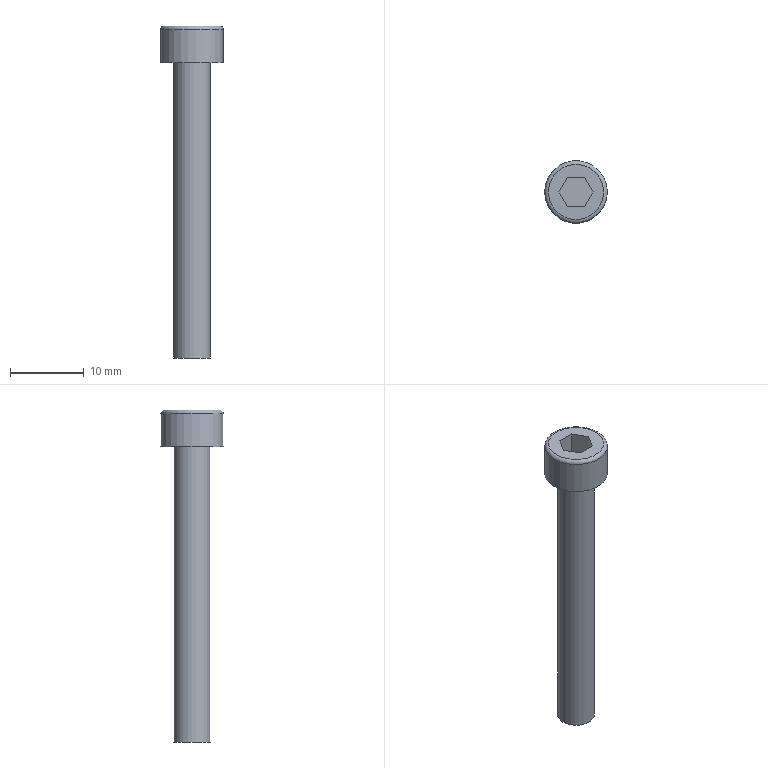Part | STEP file | Tube necking machine_id750_x_t | 1 solid | 13 faces | box 8.5 x 8.5 x 45 mm | volume 1022 mm3 | plane 10 | cylinder 2 | torus 1 | commonest cylinder face diameters 5 x1 8.5 x1
STEP:
#1=CARTESIAN_POINT('',(0.,0.,0.));
#2=DIRECTION('',(0.,0.,1.));
#3=DIRECTION('',(1.,0.,0.));
#4=AXIS2_PLACEMENT_3D('',#1,#2,#3);
#5=CARTESIAN_POINT('',(-17.75,-335.,207.));
#6=VERTEX_POINT('',#5);
#7=CARTESIAN_POINT('',(-14.,-335.,207.));
#8=DIRECTION('',(0.,0.,1.));
#9=DIRECTION('',(-1.,0.,0.));
#10=AXIS2_PLACEMENT_3D('',#7,#8,#9);
#11=CIRCLE('',#10,3.75);
#12=CARTESIAN_POINT('',(-9.75,-335.,207.));
#13=DIRECTION('',(0.,0.,-1.));
#14=DIRECTION('',(-1.,0.,0.));
#15=AXIS2_PLACEMENT_3D('',#12,#13,#14);
#16=PLANE('',#15);
#17=CARTESIAN_POINT('',(8.,0.));
#18=CARTESIAN_POINT('',(8.,-6.495));
#19=CARTESIAN_POINT('',(2.375,-3.248));
#20=CARTESIAN_POINT('',(-3.25,0.));
#21=CARTESIAN_POINT('',(2.375,3.248));
#22=CARTESIAN_POINT('',(8.,6.495));
#23=CARTESIAN_POINT('',(8.,0.));
#24=(BOUNDED_CURVE()B_SPLINE_CURVE(2,(#17,#18,#19,#20,#21,#22,#23),.UNSPECIFIED.,.T.,.F.)B_SPLINE_CURVE_WITH_KNOTS((1,2,2,2,2,1),(-2.094,0.,2.094,4.189,6.283,8.378),.UNSPECIFIED.)CURVE()GEOMETRIC_REPRESENTATION_ITEM()RATIONAL_B_SPLINE_CURVE((1.,0.5,1.,0.5,1.,0.5,1.))REPRESENTATION_ITEM(''));
#25=(GEOMETRIC_REPRESENTATION_CONTEXT(2)PARAMETRIC_REPRESENTATION_CONTEXT()REPRESENTATION_CONTEXT('',''));
#26=DEFINITIONAL_REPRESENTATION('',(#24),#25);
#27=PCURVE('',#16,#26);
#28=CARTESIAN_POINT('',(-14.,-335.,206.5));
#29=DIRECTION('',(0.,0.,-1.));
#30=DIRECTION('',(-1.,0.,0.));
#31=AXIS2_PLACEMENT_3D('',#28,#29,#30);
#32=TOROIDAL_SURFACE('',#31,3.75,0.5);
#33=CARTESIAN_POINT('',(6.283,4.712));
#34=DIRECTION('',(-1.,0.));
#35=VECTOR('',#34,1.);
#36=LINE('',#33,#35);
#37=(GEOMETRIC_REPRESENTATION_CONTEXT(2)PARAMETRIC_REPRESENTATION_CONTEXT()REPRESENTATION_CONTEXT('',''));
#38=DEFINITIONAL_REPRESENTATION('',(#36),#37);
#39=PCURVE('',#32,#38);
#40=SURFACE_CURVE('',#11,(#27,#39),.PCURVE_S1.);
#41=EDGE_CURVE('',#6,#6,#40,.T.);
#42=ORIENTED_EDGE('',*,*,#41,.T.);
#43=EDGE_LOOP('',(#42));
#44=FACE_BOUND('',#43,.T.);
#45=CARTESIAN_POINT('',(-15.155,-333.,207.));
#46=VERTEX_POINT('',#45);
#47=CARTESIAN_POINT('',(-12.845,-333.,207.));
#48=VERTEX_POINT('',#47);
#49=CARTESIAN_POINT('',(-15.155,-333.,207.));
#50=DIRECTION('',(1.,0.,0.));
#51=VECTOR('',#50,1.);
#52=LINE('',#49,#51);
#53=CARTESIAN_POINT('',(5.405,2.));
#54=DIRECTION('',(-1.,0.));
#55=VECTOR('',#54,1.);
#56=LINE('',#53,#55);
#57=(GEOMETRIC_REPRESENTATION_CONTEXT(2)PARAMETRIC_REPRESENTATION_CONTEXT()REPRESENTATION_CONTEXT('',''));
#58=DEFINITIONAL_REPRESENTATION('',(#56),#57);
#59=PCURVE('',#16,#58);
#60=CARTESIAN_POINT('',(-15.155,-333.,203.7));
#61=DIRECTION('',(0.,-1.,0.));
#62=DIRECTION('',(1.,0.,0.));
#63=AXIS2_PLACEMENT_3D('',#60,#61,#62);
#64=PLANE('',#63);
#65=CARTESIAN_POINT('',(0.,3.3));
#66=DIRECTION('',(1.,0.));
#67=VECTOR('',#66,1.);
#68=LINE('',#65,#67);
#69=(GEOMETRIC_REPRESENTATION_CONTEXT(2)PARAMETRIC_REPRESENTATION_CONTEXT()REPRESENTATION_CONTEXT('',''));
#70=DEFINITIONAL_REPRESENTATION('',(#68),#69);
#71=PCURVE('',#64,#70);
#72=SURFACE_CURVE('',#52,(#59,#71),.PCURVE_S1.);
#73=EDGE_CURVE('',#46,#48,#72,.T.);
#74=ORIENTED_EDGE('',*,*,#73,.T.);
#75=CARTESIAN_POINT('',(-11.691,-335.,207.));
#76=VERTEX_POINT('',#75);
#77=CARTESIAN_POINT('',(-12.845,-333.,207.));
#78=DIRECTION('',(0.5,-0.866,0.));
#79=VECTOR('',#78,1.);
#80=LINE('',#77,#79);
#81=CARTESIAN_POINT('',(3.095,2.));
#82=DIRECTION('',(-0.5,-0.866));
#83=VECTOR('',#82,1.);
#84=LINE('',#81,#83);
#85=(GEOMETRIC_REPRESENTATION_CONTEXT(2)PARAMETRIC_REPRESENTATION_CONTEXT()REPRESENTATION_CONTEXT('',''));
#86=DEFINITIONAL_REPRESENTATION('',(#84),#85);
#87=PCURVE('',#16,#86);
#88=CARTESIAN_POINT('',(-12.845,-333.,203.7));
#89=DIRECTION('',(-0.866,-0.5,0.));
#90=DIRECTION('',(0.5,-0.866,0.));
#91=AXIS2_PLACEMENT_3D('',#88,#89,#90);
#92=PLANE('',#91);
#93=CARTESIAN_POINT('',(0.,3.3));
#94=DIRECTION('',(1.,0.));
#95=VECTOR('',#94,1.);
#96=LINE('',#93,#95);
#97=(GEOMETRIC_REPRESENTATION_CONTEXT(2)PARAMETRIC_REPRESENTATION_CONTEXT()REPRESENTATION_CONTEXT('',''));
#98=DEFINITIONAL_REPRESENTATION('',(#96),#97);
#99=PCURVE('',#92,#98);
#100=SURFACE_CURVE('',#80,(#87,#99),.PCURVE_S1.);
#101=EDGE_CURVE('',#48,#76,#100,.T.);
#102=ORIENTED_EDGE('',*,*,#101,.T.);
#103=CARTESIAN_POINT('',(-12.845,-337.,207.));
#104=VERTEX_POINT('',#103);
#105=CARTESIAN_POINT('',(-11.691,-335.,207.));
#106=DIRECTION('',(-0.5,-0.866,0.));
#107=VECTOR('',#106,1.);
#108=LINE('',#105,#107);
#109=CARTESIAN_POINT('',(1.941,0.));
#110=DIRECTION('',(0.5,-0.866));
#111=VECTOR('',#110,1.);
#112=LINE('',#109,#111);
#113=(GEOMETRIC_REPRESENTATION_CONTEXT(2)PARAMETRIC_REPRESENTATION_CONTEXT()REPRESENTATION_CONTEXT('',''));
#114=DEFINITIONAL_REPRESENTATION('',(#112),#113);
#115=PCURVE('',#16,#114);
#116=CARTESIAN_POINT('',(-11.691,-335.,203.7));
#117=DIRECTION('',(-0.866,0.5,0.));
#118=DIRECTION('',(-0.5,-0.866,0.));
#119=AXIS2_PLACEMENT_3D('',#116,#117,#118);
#120=PLANE('',#119);
#121=CARTESIAN_POINT('',(0.,3.3));
#122=DIRECTION('',(1.,0.));
#123=VECTOR('',#122,1.);
#124=LINE('',#121,#123);
#125=(GEOMETRIC_REPRESENTATION_CONTEXT(2)PARAMETRIC_REPRESENTATION_CONTEXT()REPRESENTATION_CONTEXT('',''));
#126=DEFINITIONAL_REPRESENTATION('',(#124),#125);
#127=PCURVE('',#120,#126);
#128=SURFACE_CURVE('',#108,(#115,#127),.PCURVE_S1.);
#129=EDGE_CURVE('',#76,#104,#128,.T.);
#130=ORIENTED_EDGE('',*,*,#129,.T.);
#131=CARTESIAN_POINT('',(-15.155,-337.,207.));
#132=VERTEX_POINT('',#131);
#133=CARTESIAN_POINT('',(-12.845,-337.,207.));
#134=DIRECTION('',(-1.,0.,0.));
#135=VECTOR('',#134,1.);
#136=LINE('',#133,#135);
#137=CARTESIAN_POINT('',(3.095,-2.));
#138=DIRECTION('',(1.,0.));
#139=VECTOR('',#138,1.);
#140=LINE('',#137,#139);
#141=(GEOMETRIC_REPRESENTATION_CONTEXT(2)PARAMETRIC_REPRESENTATION_CONTEXT()REPRESENTATION_CONTEXT('',''));
#142=DEFINITIONAL_REPRESENTATION('',(#140),#141);
#143=PCURVE('',#16,#142);
#144=CARTESIAN_POINT('',(-12.845,-337.,203.7));
#145=DIRECTION('',(0.,1.,0.));
#146=DIRECTION('',(-1.,0.,0.));
#147=AXIS2_PLACEMENT_3D('',#144,#145,#146);
#148=PLANE('',#147);
#149=CARTESIAN_POINT('',(0.,3.3));
#150=DIRECTION('',(1.,0.));
#151=VECTOR('',#150,1.);
#152=LINE('',#149,#151);
#153=(GEOMETRIC_REPRESENTATION_CONTEXT(2)PARAMETRIC_REPRESENTATION_CONTEXT()REPRESENTATION_CONTEXT('',''));
#154=DEFINITIONAL_REPRESENTATION('',(#152),#153);
#155=PCURVE('',#148,#154);
#156=SURFACE_CURVE('',#136,(#143,#155),.PCURVE_S1.);
#157=EDGE_CURVE('',#104,#132,#156,.T.);
#158=ORIENTED_EDGE('',*,*,#157,.T.);
#159=CARTESIAN_POINT('',(-16.309,-335.,207.));
#160=VERTEX_POINT('',#159);
#161=CARTESIAN_POINT('',(-15.155,-337.,207.));
#162=DIRECTION('',(-0.5,0.866,0.));
#163=VECTOR('',#162,1.);
#164=LINE('',#161,#163);
#165=CARTESIAN_POINT('',(5.405,-2.));
#166=DIRECTION('',(0.5,0.866));
#167=VECTOR('',#166,1.);
#168=LINE('',#165,#167);
#169=(GEOMETRIC_REPRESENTATION_CONTEXT(2)PARAMETRIC_REPRESENTATION_CONTEXT()REPRESENTATION_CONTEXT('',''));
#170=DEFINITIONAL_REPRESENTATION('',(#168),#169);
#171=PCURVE('',#16,#170);
#172=CARTESIAN_POINT('',(-15.155,-337.,203.7));
#173=DIRECTION('',(0.866,0.5,0.));
#174=DIRECTION('',(-0.5,0.866,0.));
#175=AXIS2_PLACEMENT_3D('',#172,#173,#174);
#176=PLANE('',#175);
#177=CARTESIAN_POINT('',(0.,3.3));
#178=DIRECTION('',(1.,0.));
#179=VECTOR('',#178,1.);
#180=LINE('',#177,#179);
#181=(GEOMETRIC_REPRESENTATION_CONTEXT(2)PARAMETRIC_REPRESENTATION_CONTEXT()REPRESENTATION_CONTEXT('',''));
#182=DEFINITIONAL_REPRESENTATION('',(#180),#181);
#183=PCURVE('',#176,#182);
#184=SURFACE_CURVE('',#164,(#171,#183),.PCURVE_S1.);
#185=EDGE_CURVE('',#132,#160,#184,.T.);
#186=ORIENTED_EDGE('',*,*,#185,.T.);
#187=CARTESIAN_POINT('',(-16.309,-335.,207.));
#188=DIRECTION('',(0.5,0.866,0.));
#189=VECTOR('',#188,1.);
#190=LINE('',#187,#189);
#191=CARTESIAN_POINT('',(6.559,0.));
#192=DIRECTION('',(-0.5,0.866));
#193=VECTOR('',#192,1.);
#194=LINE('',#191,#193);
#195=(GEOMETRIC_REPRESENTATION_CONTEXT(2)PARAMETRIC_REPRESENTATION_CONTEXT()REPRESENTATION_CONTEXT('',''));
#196=DEFINITIONAL_REPRESENTATION('',(#194),#195);
#197=PCURVE('',#16,#196);
#198=CARTESIAN_POINT('',(-16.309,-335.,203.7));
#199=DIRECTION('',(0.866,-0.5,0.));
#200=DIRECTION('',(0.5,0.866,0.));
#201=AXIS2_PLACEMENT_3D('',#198,#199,#200);
#202=PLANE('',#201);
#203=CARTESIAN_POINT('',(0.,3.3));
#204=DIRECTION('',(1.,0.));
#205=VECTOR('',#204,1.);
#206=LINE('',#203,#205);
#207=(GEOMETRIC_REPRESENTATION_CONTEXT(2)PARAMETRIC_REPRESENTATION_CONTEXT()REPRESENTATION_CONTEXT('',''));
#208=DEFINITIONAL_REPRESENTATION('',(#206),#207);
#209=PCURVE('',#202,#208);
#210=SURFACE_CURVE('',#190,(#197,#209),.PCURVE_S1.);
#211=EDGE_CURVE('',#160,#46,#210,.T.);
#212=ORIENTED_EDGE('',*,*,#211,.T.);
#213=EDGE_LOOP('',(#74,#102,#130,#158,#186,#212));
#214=FACE_BOUND('',#213,.T.);
#215=ADVANCED_FACE('',(#44,#214),#16,.F.);
#216=CARTESIAN_POINT('',(-18.25,-335.,206.5));
#217=VERTEX_POINT('',#216);
#218=CARTESIAN_POINT('',(-9.75,-335.,206.5));
#219=VERTEX_POINT('',#218);
#220=CARTESIAN_POINT('',(-14.,-335.,206.5));
#221=DIRECTION('',(0.,0.,-1.));
#222=DIRECTION('',(-1.,0.,0.));
#223=AXIS2_PLACEMENT_3D('',#220,#221,#222);
#224=CIRCLE('',#223,4.25);
#225=CARTESIAN_POINT('',(-14.,-335.,203.1));
#226=DIRECTION('',(0.,0.,1.));
#227=DIRECTION('',(1.,0.,0.));
#228=AXIS2_PLACEMENT_3D('',#225,#226,#227);
#229=CYLINDRICAL_SURFACE('',#228,4.25);
#230=CARTESIAN_POINT('',(3.142,3.4));
#231=DIRECTION('',(-1.,0.));
#232=VECTOR('',#231,1.);
#233=LINE('',#230,#232);
#234=(GEOMETRIC_REPRESENTATION_CONTEXT(2)PARAMETRIC_REPRESENTATION_CONTEXT()REPRESENTATION_CONTEXT('',''));
#235=DEFINITIONAL_REPRESENTATION('',(#233),#234);
#236=PCURVE('',#229,#235);
#237=CARTESIAN_POINT('',(0.,6.283));
#238=DIRECTION('',(1.,0.));
#239=VECTOR('',#238,1.);
#240=LINE('',#237,#239);
#241=(GEOMETRIC_REPRESENTATION_CONTEXT(2)PARAMETRIC_REPRESENTATION_CONTEXT()REPRESENTATION_CONTEXT('',''));
#242=DEFINITIONAL_REPRESENTATION('',(#240),#241);
#243=PCURVE('',#32,#242);
#244=SURFACE_CURVE('',#224,(#236,#243),.PCURVE_S1.);
#245=EDGE_CURVE('',#217,#219,#244,.T.);
#246=ORIENTED_EDGE('',*,*,#245,.T.);
#247=CARTESIAN_POINT('',(-9.75,-335.,202.));
#248=VERTEX_POINT('',#247);
#249=CARTESIAN_POINT('',(-9.75,-335.,202.));
#250=CARTESIAN_POINT('',(-9.75,-335.,206.5));
#251=B_SPLINE_CURVE_WITH_KNOTS('',1,(#249,#250),.UNSPECIFIED.,.F.,.F.,(2,2),(-1.1,3.4),.PIECEWISE_BEZIER_KNOTS.);
#252=CARTESIAN_POINT('',(0.,0.));
#253=DIRECTION('',(0.,1.));
#254=VECTOR('',#253,1.);
#255=LINE('',#252,#254);
#256=(GEOMETRIC_REPRESENTATION_CONTEXT(2)PARAMETRIC_REPRESENTATION_CONTEXT()REPRESENTATION_CONTEXT('',''));
#257=DEFINITIONAL_REPRESENTATION('',(#255),#256);
#258=PCURVE('',#229,#257);
#259=CARTESIAN_POINT('',(6.283,0.));
#260=DIRECTION('',(0.,1.));
#261=VECTOR('',#260,1.);
#262=LINE('',#259,#261);
#263=(GEOMETRIC_REPRESENTATION_CONTEXT(2)PARAMETRIC_REPRESENTATION_CONTEXT()REPRESENTATION_CONTEXT('',''));
#264=DEFINITIONAL_REPRESENTATION('',(#262),#263);
#265=PCURVE('',#229,#264);
#266=SEAM_CURVE('',#251,(#258,#265),.PCURVE_S1.);
#267=EDGE_CURVE('',#248,#219,#266,.T.);
#268=ORIENTED_EDGE('',*,*,#267,.F.);
#269=CARTESIAN_POINT('',(-14.,-335.,202.));
#270=DIRECTION('',(0.,0.,1.));
#271=DIRECTION('',(1.,0.,0.));
#272=AXIS2_PLACEMENT_3D('',#269,#270,#271);
#273=CIRCLE('',#272,4.25);
#274=CARTESIAN_POINT('',(0.,-1.1));
#275=DIRECTION('',(1.,0.));
#276=VECTOR('',#275,1.);
#277=LINE('',#274,#276);
#278=(GEOMETRIC_REPRESENTATION_CONTEXT(2)PARAMETRIC_REPRESENTATION_CONTEXT()REPRESENTATION_CONTEXT('',''));
#279=DEFINITIONAL_REPRESENTATION('',(#277),#278);
#280=PCURVE('',#229,#279);
#281=CARTESIAN_POINT('',(-11.5,-335.,202.));
#282=DIRECTION('',(0.,0.,1.));
#283=DIRECTION('',(1.,0.,0.));
#284=AXIS2_PLACEMENT_3D('',#281,#282,#283);
#285=PLANE('',#284);
#286=CARTESIAN_POINT('',(-2.5,0.));
#287=DIRECTION('',(1.,0.));
#288=AXIS2_PLACEMENT_2D('',#286,#287);
#289=CIRCLE('',#288,4.25);
#290=(GEOMETRIC_REPRESENTATION_CONTEXT(2)PARAMETRIC_REPRESENTATION_CONTEXT()REPRESENTATION_CONTEXT('',''));
#291=DEFINITIONAL_REPRESENTATION('',(#289),#290);
#292=PCURVE('',#285,#291);
#293=SURFACE_CURVE('',#273,(#280,#292),.PCURVE_S1.);
#294=EDGE_CURVE('',#248,#248,#293,.T.);
#295=ORIENTED_EDGE('',*,*,#294,.T.);
#296=ORIENTED_EDGE('',*,*,#267,.T.);
#297=CARTESIAN_POINT('',(-14.,-335.,206.5));
#298=DIRECTION('',(0.,0.,-1.));
#299=DIRECTION('',(-1.,0.,0.));
#300=AXIS2_PLACEMENT_3D('',#297,#298,#299);
#301=CIRCLE('',#300,4.25);
#302=CARTESIAN_POINT('',(9.425,3.4));
#303=DIRECTION('',(-1.,0.));
#304=VECTOR('',#303,1.);
#305=LINE('',#302,#304);
#306=(GEOMETRIC_REPRESENTATION_CONTEXT(2)PARAMETRIC_REPRESENTATION_CONTEXT()REPRESENTATION_CONTEXT('',''));
#307=DEFINITIONAL_REPRESENTATION('',(#305),#306);
#308=PCURVE('',#229,#307);
#309=CARTESIAN_POINT('',(0.,6.283));
#310=DIRECTION('',(1.,0.));
#311=VECTOR('',#310,1.);
#312=LINE('',#309,#311);
#313=(GEOMETRIC_REPRESENTATION_CONTEXT(2)PARAMETRIC_REPRESENTATION_CONTEXT()REPRESENTATION_CONTEXT('',''));
#314=DEFINITIONAL_REPRESENTATION('',(#312),#313);
#315=PCURVE('',#32,#314);
#316=SURFACE_CURVE('',#301,(#308,#315),.PCURVE_S1.);
#317=EDGE_CURVE('',#219,#217,#316,.T.);
#318=ORIENTED_EDGE('',*,*,#317,.T.);
#319=EDGE_LOOP('',(#246,#268,#295,#296,#318));
#320=FACE_BOUND('',#319,.T.);
#321=ADVANCED_FACE('',(#320),#229,.T.);
#322=ORIENTED_EDGE('',*,*,#294,.F.);
#323=EDGE_LOOP('',(#322));
#324=FACE_BOUND('',#323,.T.);
#325=CARTESIAN_POINT('',(-11.5,-335.,202.));
#326=VERTEX_POINT('',#325);
#327=CARTESIAN_POINT('',(-14.,-335.,202.));
#328=DIRECTION('',(0.,0.,1.));
#329=DIRECTION('',(1.,0.,0.));
#330=AXIS2_PLACEMENT_3D('',#327,#328,#329);
#331=CIRCLE('',#330,2.5);
#332=CARTESIAN_POINT('',(-2.5,0.));
#333=DIRECTION('',(1.,0.));
#334=AXIS2_PLACEMENT_2D('',#332,#333);
#335=CIRCLE('',#334,2.5);
#336=(GEOMETRIC_REPRESENTATION_CONTEXT(2)PARAMETRIC_REPRESENTATION_CONTEXT()REPRESENTATION_CONTEXT('',''));
#337=DEFINITIONAL_REPRESENTATION('',(#335),#336);
#338=PCURVE('',#285,#337);
#339=CARTESIAN_POINT('',(-14.,-335.,203.1));
#340=DIRECTION('',(0.,0.,1.));
#341=DIRECTION('',(1.,0.,0.));
#342=AXIS2_PLACEMENT_3D('',#339,#340,#341);
#343=CYLINDRICAL_SURFACE('',#342,2.5);
#344=CARTESIAN_POINT('',(0.,-1.1));
#345=DIRECTION('',(1.,0.));
#346=VECTOR('',#345,1.);
#347=LINE('',#344,#346);
#348=(GEOMETRIC_REPRESENTATION_CONTEXT(2)PARAMETRIC_REPRESENTATION_CONTEXT()REPRESENTATION_CONTEXT('',''));
#349=DEFINITIONAL_REPRESENTATION('',(#347),#348);
#350=PCURVE('',#343,#349);
#351=SURFACE_CURVE('',#331,(#338,#350),.PCURVE_S1.);
#352=EDGE_CURVE('',#326,#326,#351,.T.);
#353=ORIENTED_EDGE('',*,*,#352,.T.);
#354=EDGE_LOOP('',(#353));
#355=FACE_BOUND('',#354,.T.);
#356=ADVANCED_FACE('',(#324,#355),#285,.F.);
#357=ORIENTED_EDGE('',*,*,#352,.F.);
#358=CARTESIAN_POINT('',(-11.5,-335.,162.));
#359=VERTEX_POINT('',#358);
#360=CARTESIAN_POINT('',(-11.5,-335.,162.));
#361=CARTESIAN_POINT('',(-11.5,-335.,202.));
#362=B_SPLINE_CURVE_WITH_KNOTS('',1,(#360,#361),.UNSPECIFIED.,.F.,.F.,(2,2),(-41.1,-1.1),.PIECEWISE_BEZIER_KNOTS.);
#363=CARTESIAN_POINT('',(0.,0.));
#364=DIRECTION('',(0.,1.));
#365=VECTOR('',#364,1.);
#366=LINE('',#363,#365);
#367=(GEOMETRIC_REPRESENTATION_CONTEXT(2)PARAMETRIC_REPRESENTATION_CONTEXT()REPRESENTATION_CONTEXT('',''));
#368=DEFINITIONAL_REPRESENTATION('',(#366),#367);
#369=PCURVE('',#343,#368);
#370=CARTESIAN_POINT('',(6.283,0.));
#371=DIRECTION('',(0.,1.));
#372=VECTOR('',#371,1.);
#373=LINE('',#370,#372);
#374=(GEOMETRIC_REPRESENTATION_CONTEXT(2)PARAMETRIC_REPRESENTATION_CONTEXT()REPRESENTATION_CONTEXT('',''));
#375=DEFINITIONAL_REPRESENTATION('',(#373),#374);
#376=PCURVE('',#343,#375);
#377=SEAM_CURVE('',#362,(#369,#376),.PCURVE_S1.);
#378=EDGE_CURVE('',#359,#326,#377,.T.);
#379=ORIENTED_EDGE('',*,*,#378,.F.);
#380=CARTESIAN_POINT('',(-14.,-335.,162.));
#381=DIRECTION('',(0.,0.,1.));
#382=DIRECTION('',(1.,0.,0.));
#383=AXIS2_PLACEMENT_3D('',#380,#381,#382);
#384=CIRCLE('',#383,2.5);
#385=CARTESIAN_POINT('',(0.,-41.1));
#386=DIRECTION('',(1.,0.));
#387=VECTOR('',#386,1.);
#388=LINE('',#385,#387);
#389=(GEOMETRIC_REPRESENTATION_CONTEXT(2)PARAMETRIC_REPRESENTATION_CONTEXT()REPRESENTATION_CONTEXT('',''));
#390=DEFINITIONAL_REPRESENTATION('',(#388),#389);
#391=PCURVE('',#343,#390);
#392=CARTESIAN_POINT('',(-14.,-335.,162.));
#393=DIRECTION('',(0.,0.,1.));
#394=DIRECTION('',(1.,0.,0.));
#395=AXIS2_PLACEMENT_3D('',#392,#393,#394);
#396=PLANE('',#395);
#397=CARTESIAN_POINT('',(0.,0.));
#398=DIRECTION('',(1.,0.));
#399=AXIS2_PLACEMENT_2D('',#397,#398);
#400=CIRCLE('',#399,2.5);
#401=(GEOMETRIC_REPRESENTATION_CONTEXT(2)PARAMETRIC_REPRESENTATION_CONTEXT()REPRESENTATION_CONTEXT('',''));
#402=DEFINITIONAL_REPRESENTATION('',(#400),#401);
#403=PCURVE('',#396,#402);
#404=SURFACE_CURVE('',#384,(#391,#403),.PCURVE_S1.);
#405=EDGE_CURVE('',#359,#359,#404,.T.);
#406=ORIENTED_EDGE('',*,*,#405,.T.);
#407=ORIENTED_EDGE('',*,*,#378,.T.);
#408=EDGE_LOOP('',(#357,#379,#406,#407));
#409=FACE_BOUND('',#408,.T.);
#410=ADVANCED_FACE('',(#409),#343,.T.);
#411=ORIENTED_EDGE('',*,*,#405,.F.);
#412=EDGE_LOOP('',(#411));
#413=FACE_BOUND('',#412,.T.);
#414=ADVANCED_FACE('',(#413),#396,.F.);
#415=ORIENTED_EDGE('',*,*,#73,.F.);
#416=CARTESIAN_POINT('',(-15.155,-333.,203.7));
#417=VERTEX_POINT('',#416);
#418=CARTESIAN_POINT('',(-15.155,-333.,203.7));
#419=DIRECTION('',(0.,0.,-1.));
#420=VECTOR('',#419,1.);
#421=LINE('',#418,#420);
#422=CARTESIAN_POINT('',(0.,0.));
#423=DIRECTION('',(0.,-1.));
#424=VECTOR('',#423,1.);
#425=LINE('',#422,#424);
#426=(GEOMETRIC_REPRESENTATION_CONTEXT(2)PARAMETRIC_REPRESENTATION_CONTEXT()REPRESENTATION_CONTEXT('',''));
#427=DEFINITIONAL_REPRESENTATION('',(#425),#426);
#428=PCURVE('',#64,#427);
#429=CARTESIAN_POINT('',(2.309,0.));
#430=DIRECTION('',(0.,-1.));
#431=VECTOR('',#430,1.);
#432=LINE('',#429,#431);
#433=(GEOMETRIC_REPRESENTATION_CONTEXT(2)PARAMETRIC_REPRESENTATION_CONTEXT()REPRESENTATION_CONTEXT('',''));
#434=DEFINITIONAL_REPRESENTATION('',(#432),#433);
#435=PCURVE('',#202,#434);
#436=SURFACE_CURVE('',#421,(#428,#435),.PCURVE_S1.);
#437=EDGE_CURVE('',#46,#417,#436,.T.);
#438=ORIENTED_EDGE('',*,*,#437,.T.);
#439=CARTESIAN_POINT('',(-12.845,-333.,203.7));
#440=VERTEX_POINT('',#439);
#441=CARTESIAN_POINT('',(-15.155,-333.,203.7));
#442=DIRECTION('',(-1.,0.,0.));
#443=VECTOR('',#442,1.);
#444=LINE('',#441,#443);
#445=CARTESIAN_POINT('',(0.,0.));
#446=DIRECTION('',(-1.,0.));
#447=VECTOR('',#446,1.);
#448=LINE('',#445,#447);
#449=(GEOMETRIC_REPRESENTATION_CONTEXT(2)PARAMETRIC_REPRESENTATION_CONTEXT()REPRESENTATION_CONTEXT('',''));
#450=DEFINITIONAL_REPRESENTATION('',(#448),#449);
#451=PCURVE('',#64,#450);
#452=CARTESIAN_POINT('',(-14.,-335.,203.7));
#453=DIRECTION('',(0.,0.,-1.));
#454=DIRECTION('',(-1.,0.,0.));
#455=AXIS2_PLACEMENT_3D('',#452,#453,#454);
#456=PLANE('',#455);
#457=CARTESIAN_POINT('',(1.155,2.));
#458=DIRECTION('',(1.,0.));
#459=VECTOR('',#458,1.);
#460=LINE('',#457,#459);
#461=(GEOMETRIC_REPRESENTATION_CONTEXT(2)PARAMETRIC_REPRESENTATION_CONTEXT()REPRESENTATION_CONTEXT('',''));
#462=DEFINITIONAL_REPRESENTATION('',(#460),#461);
#463=PCURVE('',#456,#462);
#464=SURFACE_CURVE('',#444,(#451,#463),.PCURVE_S1.);
#465=EDGE_CURVE('',#440,#417,#464,.T.);
#466=ORIENTED_EDGE('',*,*,#465,.F.);
#467=CARTESIAN_POINT('',(-12.845,-333.,203.7));
#468=DIRECTION('',(0.,0.,-1.));
#469=VECTOR('',#468,1.);
#470=LINE('',#467,#469);
#471=CARTESIAN_POINT('',(2.309,0.));
#472=DIRECTION('',(0.,-1.));
#473=VECTOR('',#472,1.);
#474=LINE('',#471,#473);
#475=(GEOMETRIC_REPRESENTATION_CONTEXT(2)PARAMETRIC_REPRESENTATION_CONTEXT()REPRESENTATION_CONTEXT('',''));
#476=DEFINITIONAL_REPRESENTATION('',(#474),#475);
#477=PCURVE('',#64,#476);
#478=CARTESIAN_POINT('',(0.,0.));
#479=DIRECTION('',(0.,-1.));
#480=VECTOR('',#479,1.);
#481=LINE('',#478,#480);
#482=(GEOMETRIC_REPRESENTATION_CONTEXT(2)PARAMETRIC_REPRESENTATION_CONTEXT()REPRESENTATION_CONTEXT('',''));
#483=DEFINITIONAL_REPRESENTATION('',(#481),#482);
#484=PCURVE('',#92,#483);
#485=SURFACE_CURVE('',#470,(#477,#484),.PCURVE_S1.);
#486=EDGE_CURVE('',#48,#440,#485,.T.);
#487=ORIENTED_EDGE('',*,*,#486,.F.);
#488=EDGE_LOOP('',(#415,#438,#466,#487));
#489=FACE_BOUND('',#488,.T.);
#490=ADVANCED_FACE('',(#489),#64,.T.);
#491=ORIENTED_EDGE('',*,*,#101,.F.);
#492=ORIENTED_EDGE('',*,*,#486,.T.);
#493=CARTESIAN_POINT('',(-11.691,-335.,203.7));
#494=VERTEX_POINT('',#493);
#495=CARTESIAN_POINT('',(-12.845,-333.,203.7));
#496=DIRECTION('',(-0.5,0.866,0.));
#497=VECTOR('',#496,1.);
#498=LINE('',#495,#497);
#499=CARTESIAN_POINT('',(0.,0.));
#500=DIRECTION('',(-1.,0.));
#501=VECTOR('',#500,1.);
#502=LINE('',#499,#501);
#503=(GEOMETRIC_REPRESENTATION_CONTEXT(2)PARAMETRIC_REPRESENTATION_CONTEXT()REPRESENTATION_CONTEXT('',''));
#504=DEFINITIONAL_REPRESENTATION('',(#502),#503);
#505=PCURVE('',#92,#504);
#506=CARTESIAN_POINT('',(-1.155,2.));
#507=DIRECTION('',(0.5,0.866));
#508=VECTOR('',#507,1.);
#509=LINE('',#506,#508);
#510=(GEOMETRIC_REPRESENTATION_CONTEXT(2)PARAMETRIC_REPRESENTATION_CONTEXT()REPRESENTATION_CONTEXT('',''));
#511=DEFINITIONAL_REPRESENTATION('',(#509),#510);
#512=PCURVE('',#456,#511);
#513=SURFACE_CURVE('',#498,(#505,#512),.PCURVE_S1.);
#514=EDGE_CURVE('',#494,#440,#513,.T.);
#515=ORIENTED_EDGE('',*,*,#514,.F.);
#516=CARTESIAN_POINT('',(-11.691,-335.,203.7));
#517=DIRECTION('',(0.,0.,-1.));
#518=VECTOR('',#517,1.);
#519=LINE('',#516,#518);
#520=CARTESIAN_POINT('',(2.309,0.));
#521=DIRECTION('',(0.,-1.));
#522=VECTOR('',#521,1.);
#523=LINE('',#520,#522);
#524=(GEOMETRIC_REPRESENTATION_CONTEXT(2)PARAMETRIC_REPRESENTATION_CONTEXT()REPRESENTATION_CONTEXT('',''));
#525=DEFINITIONAL_REPRESENTATION('',(#523),#524);
#526=PCURVE('',#92,#525);
#527=CARTESIAN_POINT('',(0.,0.));
#528=DIRECTION('',(0.,-1.));
#529=VECTOR('',#528,1.);
#530=LINE('',#527,#529);
#531=(GEOMETRIC_REPRESENTATION_CONTEXT(2)PARAMETRIC_REPRESENTATION_CONTEXT()REPRESENTATION_CONTEXT('',''));
#532=DEFINITIONAL_REPRESENTATION('',(#530),#531);
#533=PCURVE('',#120,#532);
#534=SURFACE_CURVE('',#519,(#526,#533),.PCURVE_S1.);
#535=EDGE_CURVE('',#76,#494,#534,.T.);
#536=ORIENTED_EDGE('',*,*,#535,.F.);
#537=EDGE_LOOP('',(#491,#492,#515,#536));
#538=FACE_BOUND('',#537,.T.);
#539=ADVANCED_FACE('',(#538),#92,.T.);
#540=ORIENTED_EDGE('',*,*,#129,.F.);
#541=ORIENTED_EDGE('',*,*,#535,.T.);
#542=CARTESIAN_POINT('',(-12.845,-337.,203.7));
#543=VERTEX_POINT('',#542);
#544=CARTESIAN_POINT('',(-11.691,-335.,203.7));
#545=DIRECTION('',(0.5,0.866,0.));
#546=VECTOR('',#545,1.);
#547=LINE('',#544,#546);
#548=CARTESIAN_POINT('',(0.,0.));
#549=DIRECTION('',(-1.,0.));
#550=VECTOR('',#549,1.);
#551=LINE('',#548,#550);
#552=(GEOMETRIC_REPRESENTATION_CONTEXT(2)PARAMETRIC_REPRESENTATION_CONTEXT()REPRESENTATION_CONTEXT('',''));
#553=DEFINITIONAL_REPRESENTATION('',(#551),#552);
#554=PCURVE('',#120,#553);
#555=CARTESIAN_POINT('',(-2.309,0.));
#556=DIRECTION('',(-0.5,0.866));
#557=VECTOR('',#556,1.);
#558=LINE('',#555,#557);
#559=(GEOMETRIC_REPRESENTATION_CONTEXT(2)PARAMETRIC_REPRESENTATION_CONTEXT()REPRESENTATION_CONTEXT('',''));
#560=DEFINITIONAL_REPRESENTATION('',(#558),#559);
#561=PCURVE('',#456,#560);
#562=SURFACE_CURVE('',#547,(#554,#561),.PCURVE_S1.);
#563=EDGE_CURVE('',#543,#494,#562,.T.);
#564=ORIENTED_EDGE('',*,*,#563,.F.);
#565=CARTESIAN_POINT('',(-12.845,-337.,203.7));
#566=DIRECTION('',(0.,0.,-1.));
#567=VECTOR('',#566,1.);
#568=LINE('',#565,#567);
#569=CARTESIAN_POINT('',(2.309,0.));
#570=DIRECTION('',(0.,-1.));
#571=VECTOR('',#570,1.);
#572=LINE('',#569,#571);
#573=(GEOMETRIC_REPRESENTATION_CONTEXT(2)PARAMETRIC_REPRESENTATION_CONTEXT()REPRESENTATION_CONTEXT('',''));
#574=DEFINITIONAL_REPRESENTATION('',(#572),#573);
#575=PCURVE('',#120,#574);
#576=CARTESIAN_POINT('',(0.,0.));
#577=DIRECTION('',(0.,-1.));
#578=VECTOR('',#577,1.);
#579=LINE('',#576,#578);
#580=(GEOMETRIC_REPRESENTATION_CONTEXT(2)PARAMETRIC_REPRESENTATION_CONTEXT()REPRESENTATION_CONTEXT('',''));
#581=DEFINITIONAL_REPRESENTATION('',(#579),#580);
#582=PCURVE('',#148,#581);
#583=SURFACE_CURVE('',#568,(#575,#582),.PCURVE_S1.);
#584=EDGE_CURVE('',#104,#543,#583,.T.);
#585=ORIENTED_EDGE('',*,*,#584,.F.);
#586=EDGE_LOOP('',(#540,#541,#564,#585));
#587=FACE_BOUND('',#586,.T.);
#588=ADVANCED_FACE('',(#587),#120,.T.);
#589=ORIENTED_EDGE('',*,*,#157,.F.);
#590=ORIENTED_EDGE('',*,*,#584,.T.);
#591=CARTESIAN_POINT('',(-15.155,-337.,203.7));
#592=VERTEX_POINT('',#591);
#593=CARTESIAN_POINT('',(-12.845,-337.,203.7));
#594=DIRECTION('',(1.,0.,0.));
#595=VECTOR('',#594,1.);
#596=LINE('',#593,#595);
#597=CARTESIAN_POINT('',(0.,0.));
#598=DIRECTION('',(-1.,0.));
#599=VECTOR('',#598,1.);
#600=LINE('',#597,#599);
#601=(GEOMETRIC_REPRESENTATION_CONTEXT(2)PARAMETRIC_REPRESENTATION_CONTEXT()REPRESENTATION_CONTEXT('',''));
#602=DEFINITIONAL_REPRESENTATION('',(#600),#601);
#603=PCURVE('',#148,#602);
#604=CARTESIAN_POINT('',(-1.155,-2.));
#605=DIRECTION('',(-1.,0.));
#606=VECTOR('',#605,1.);
#607=LINE('',#604,#606);
#608=(GEOMETRIC_REPRESENTATION_CONTEXT(2)PARAMETRIC_REPRESENTATION_CONTEXT()REPRESENTATION_CONTEXT('',''));
#609=DEFINITIONAL_REPRESENTATION('',(#607),#608);
#610=PCURVE('',#456,#609);
#611=SURFACE_CURVE('',#596,(#603,#610),.PCURVE_S1.);
#612=EDGE_CURVE('',#592,#543,#611,.T.);
#613=ORIENTED_EDGE('',*,*,#612,.F.);
#614=CARTESIAN_POINT('',(-15.155,-337.,203.7));
#615=DIRECTION('',(0.,0.,-1.));
#616=VECTOR('',#615,1.);
#617=LINE('',#614,#616);
#618=CARTESIAN_POINT('',(2.309,0.));
#619=DIRECTION('',(0.,-1.));
#620=VECTOR('',#619,1.);
#621=LINE('',#618,#620);
#622=(GEOMETRIC_REPRESENTATION_CONTEXT(2)PARAMETRIC_REPRESENTATION_CONTEXT()REPRESENTATION_CONTEXT('',''));
#623=DEFINITIONAL_REPRESENTATION('',(#621),#622);
#624=PCURVE('',#148,#623);
#625=CARTESIAN_POINT('',(0.,0.));
#626=DIRECTION('',(0.,-1.));
#627=VECTOR('',#626,1.);
#628=LINE('',#625,#627);
#629=(GEOMETRIC_REPRESENTATION_CONTEXT(2)PARAMETRIC_REPRESENTATION_CONTEXT()REPRESENTATION_CONTEXT('',''));
#630=DEFINITIONAL_REPRESENTATION('',(#628),#629);
#631=PCURVE('',#176,#630);
#632=SURFACE_CURVE('',#617,(#624,#631),.PCURVE_S1.);
#633=EDGE_CURVE('',#132,#592,#632,.T.);
#634=ORIENTED_EDGE('',*,*,#633,.F.);
#635=EDGE_LOOP('',(#589,#590,#613,#634));
#636=FACE_BOUND('',#635,.T.);
#637=ADVANCED_FACE('',(#636),#148,.T.);
#638=ORIENTED_EDGE('',*,*,#185,.F.);
#639=ORIENTED_EDGE('',*,*,#633,.T.);
#640=CARTESIAN_POINT('',(-16.309,-335.,203.7));
#641=VERTEX_POINT('',#640);
#642=CARTESIAN_POINT('',(-15.155,-337.,203.7));
#643=DIRECTION('',(0.5,-0.866,0.));
#644=VECTOR('',#643,1.);
#645=LINE('',#642,#644);
#646=CARTESIAN_POINT('',(0.,0.));
#647=DIRECTION('',(-1.,0.));
#648=VECTOR('',#647,1.);
#649=LINE('',#646,#648);
#650=(GEOMETRIC_REPRESENTATION_CONTEXT(2)PARAMETRIC_REPRESENTATION_CONTEXT()REPRESENTATION_CONTEXT('',''));
#651=DEFINITIONAL_REPRESENTATION('',(#649),#650);
#652=PCURVE('',#176,#651);
#653=CARTESIAN_POINT('',(1.155,-2.));
#654=DIRECTION('',(-0.5,-0.866));
#655=VECTOR('',#654,1.);
#656=LINE('',#653,#655);
#657=(GEOMETRIC_REPRESENTATION_CONTEXT(2)PARAMETRIC_REPRESENTATION_CONTEXT()REPRESENTATION_CONTEXT('',''));
#658=DEFINITIONAL_REPRESENTATION('',(#656),#657);
#659=PCURVE('',#456,#658);
#660=SURFACE_CURVE('',#645,(#652,#659),.PCURVE_S1.);
#661=EDGE_CURVE('',#641,#592,#660,.T.);
#662=ORIENTED_EDGE('',*,*,#661,.F.);
#663=CARTESIAN_POINT('',(-16.309,-335.,203.7));
#664=DIRECTION('',(0.,0.,-1.));
#665=VECTOR('',#664,1.);
#666=LINE('',#663,#665);
#667=CARTESIAN_POINT('',(2.309,0.));
#668=DIRECTION('',(0.,-1.));
#669=VECTOR('',#668,1.);
#670=LINE('',#667,#669);
#671=(GEOMETRIC_REPRESENTATION_CONTEXT(2)PARAMETRIC_REPRESENTATION_CONTEXT()REPRESENTATION_CONTEXT('',''));
#672=DEFINITIONAL_REPRESENTATION('',(#670),#671);
#673=PCURVE('',#176,#672);
#674=CARTESIAN_POINT('',(0.,0.));
#675=DIRECTION('',(0.,-1.));
#676=VECTOR('',#675,1.);
#677=LINE('',#674,#676);
#678=(GEOMETRIC_REPRESENTATION_CONTEXT(2)PARAMETRIC_REPRESENTATION_CONTEXT()REPRESENTATION_CONTEXT('',''));
#679=DEFINITIONAL_REPRESENTATION('',(#677),#678);
#680=PCURVE('',#202,#679);
#681=SURFACE_CURVE('',#666,(#673,#680),.PCURVE_S1.);
#682=EDGE_CURVE('',#160,#641,#681,.T.);
#683=ORIENTED_EDGE('',*,*,#682,.F.);
#684=EDGE_LOOP('',(#638,#639,#662,#683));
#685=FACE_BOUND('',#684,.T.);
#686=ADVANCED_FACE('',(#685),#176,.T.);
#687=ORIENTED_EDGE('',*,*,#211,.F.);
#688=ORIENTED_EDGE('',*,*,#682,.T.);
#689=CARTESIAN_POINT('',(-16.309,-335.,203.7));
#690=DIRECTION('',(-0.5,-0.866,0.));
#691=VECTOR('',#690,1.);
#692=LINE('',#689,#691);
#693=CARTESIAN_POINT('',(0.,0.));
#694=DIRECTION('',(-1.,0.));
#695=VECTOR('',#694,1.);
#696=LINE('',#693,#695);
#697=(GEOMETRIC_REPRESENTATION_CONTEXT(2)PARAMETRIC_REPRESENTATION_CONTEXT()REPRESENTATION_CONTEXT('',''));
#698=DEFINITIONAL_REPRESENTATION('',(#696),#697);
#699=PCURVE('',#202,#698);
#700=CARTESIAN_POINT('',(2.309,0.));
#701=DIRECTION('',(0.5,-0.866));
#702=VECTOR('',#701,1.);
#703=LINE('',#700,#702);
#704=(GEOMETRIC_REPRESENTATION_CONTEXT(2)PARAMETRIC_REPRESENTATION_CONTEXT()REPRESENTATION_CONTEXT('',''));
#705=DEFINITIONAL_REPRESENTATION('',(#703),#704);
#706=PCURVE('',#456,#705);
#707=SURFACE_CURVE('',#692,(#699,#706),.PCURVE_S1.);
#708=EDGE_CURVE('',#417,#641,#707,.T.);
#709=ORIENTED_EDGE('',*,*,#708,.F.);
#710=ORIENTED_EDGE('',*,*,#437,.F.);
#711=EDGE_LOOP('',(#687,#688,#709,#710));
#712=FACE_BOUND('',#711,.T.);
#713=ADVANCED_FACE('',(#712),#202,.T.);
#714=ORIENTED_EDGE('',*,*,#465,.T.);
#715=ORIENTED_EDGE('',*,*,#708,.T.);
#716=ORIENTED_EDGE('',*,*,#661,.T.);
#717=ORIENTED_EDGE('',*,*,#612,.T.);
#718=ORIENTED_EDGE('',*,*,#563,.T.);
#719=ORIENTED_EDGE('',*,*,#514,.T.);
#720=EDGE_LOOP('',(#714,#715,#716,#717,#718,#719));
#721=FACE_BOUND('',#720,.T.);
#722=ADVANCED_FACE('',(#721),#456,.F.);
#723=ORIENTED_EDGE('',*,*,#245,.F.);
#724=CARTESIAN_POINT('',(-17.75,-335.,207.));
#725=CARTESIAN_POINT('',(-17.884,-335.,207.));
#726=CARTESIAN_POINT('',(-18.014,-335.,206.957));
#727=CARTESIAN_POINT('',(-18.126,-335.,206.876));
#728=CARTESIAN_POINT('',(-18.207,-335.,206.764));
#729=CARTESIAN_POINT('',(-18.25,-335.,206.634));
#730=CARTESIAN_POINT('',(-18.25,-335.,206.5));
#731=(BOUNDED_CURVE()B_SPLINE_CURVE(6,(#724,#725,#726,#727,#728,#729,#730),.UNSPECIFIED.,.F.,.F.)B_SPLINE_CURVE_WITH_KNOTS((7,7),(-1.571,0.),.PIECEWISE_BEZIER_KNOTS.)CURVE()GEOMETRIC_REPRESENTATION_ITEM()RATIONAL_B_SPLINE_CURVE((1.031,1.01,0.9979,0.994,0.9979,1.01,1.031))REPRESENTATION_ITEM(''));
#732=CARTESIAN_POINT('',(0.,6.283));
#733=DIRECTION('',(0.,1.));
#734=VECTOR('',#733,1.);
#735=LINE('',#732,#734);
#736=(GEOMETRIC_REPRESENTATION_CONTEXT(2)PARAMETRIC_REPRESENTATION_CONTEXT()REPRESENTATION_CONTEXT('',''));
#737=DEFINITIONAL_REPRESENTATION('',(#735),#736);
#738=PCURVE('',#32,#737);
#739=CARTESIAN_POINT('',(6.283,6.283));
#740=DIRECTION('',(0.,1.));
#741=VECTOR('',#740,1.);
#742=LINE('',#739,#741);
#743=(GEOMETRIC_REPRESENTATION_CONTEXT(2)PARAMETRIC_REPRESENTATION_CONTEXT()REPRESENTATION_CONTEXT('',''));
#744=DEFINITIONAL_REPRESENTATION('',(#742),#743);
#745=PCURVE('',#32,#744);
#746=SEAM_CURVE('',#731,(#738,#745),.PCURVE_S1.);
#747=EDGE_CURVE('',#6,#217,#746,.T.);
#748=ORIENTED_EDGE('',*,*,#747,.F.);
#749=ORIENTED_EDGE('',*,*,#41,.F.);
#750=ORIENTED_EDGE('',*,*,#747,.T.);
#751=ORIENTED_EDGE('',*,*,#317,.F.);
#752=EDGE_LOOP('',(#723,#748,#749,#750,#751));
#753=FACE_BOUND('',#752,.T.);
#754=ADVANCED_FACE('',(#753),#32,.T.);
#755=CLOSED_SHELL('',(#215,#321,#356,#410,#414,#490,#539,#588,#637,#686,#713,#722,#754));
#756=MANIFOLD_SOLID_BREP('',#755);
#757=(LENGTH_UNIT()NAMED_UNIT(*)SI_UNIT(.MILLI.,.METRE.));
#758=UNCERTAINTY_MEASURE_WITH_UNIT(LENGTH_MEASURE(0.000002),#757,'','');
#759=(NAMED_UNIT(*)PLANE_ANGLE_UNIT()SI_UNIT($,.RADIAN.));
#760=(NAMED_UNIT(*)SI_UNIT($,.STERADIAN.)SOLID_ANGLE_UNIT());
#761=(GEOMETRIC_REPRESENTATION_CONTEXT(3)GLOBAL_UNCERTAINTY_ASSIGNED_CONTEXT((#758))GLOBAL_UNIT_ASSIGNED_CONTEXT((#757,#759,#760))REPRESENTATION_CONTEXT('',''));
#762=ADVANCED_BREP_SHAPE_REPRESENTATION('',(#4,#756),#761);